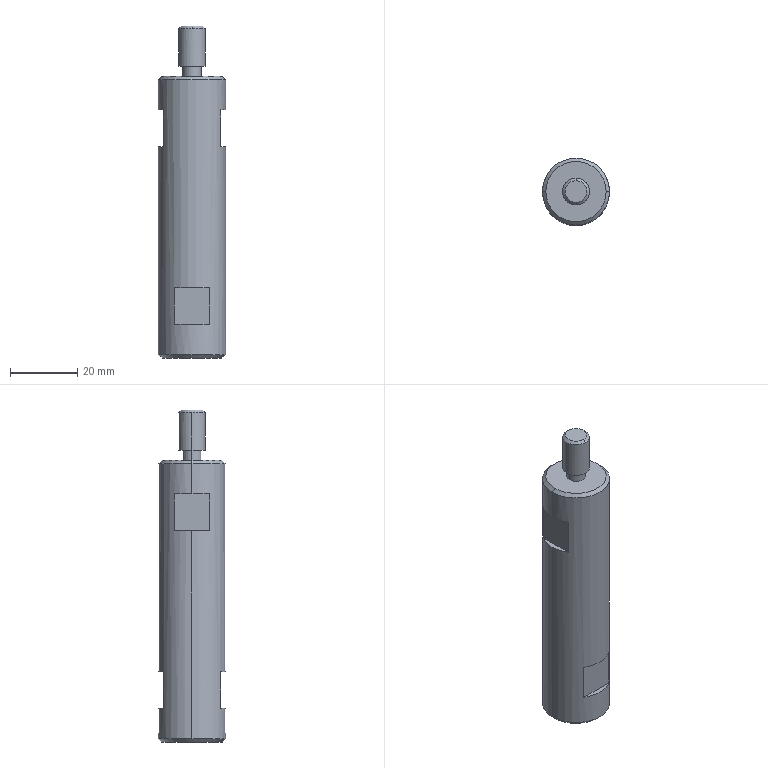Part | SolidWorks | features BaseBody 1 | 1 solid | 34 faces | box 20 x 20 x 99 mm | volume 26273 mm3 | plane 16 | cone 10 | cylinder 8 | commonest cylinder face diameters 4.917 x2 5.6 x2 8 x2 20 x2
STEP:
#1=CARTESIAN_POINT('',(-5.268,8.5,-78.));
#2=VERTEX_POINT('',#1);
#3=CARTESIAN_POINT('',(-5.268,8.5,-89.));
#4=VERTEX_POINT('',#3);
#5=CARTESIAN_POINT('',(-5.268,8.5,-50.));
#6=DIRECTION('',(0.,0.,-1.));
#7=VECTOR('',#6,1000.);
#8=LINE('',#5,#7);
#9=EDGE_CURVE('',#2,#4,#8,.T.);
#10=ORIENTED_EDGE('',*,*,#9,.T.);
#11=CARTESIAN_POINT('',(5.268,8.5,-89.));
#12=VERTEX_POINT('',#11);
#13=CARTESIAN_POINT('',(0.,0.,-89.));
#14=DIRECTION('',(0.,0.,-1.));
#15=DIRECTION('',(1.,0.,0.));
#16=AXIS2_PLACEMENT_3D('',#13,#14,#15);
#17=CIRCLE('',#16,10.);
#18=EDGE_CURVE('',#4,#12,#17,.T.);
#19=ORIENTED_EDGE('',*,*,#18,.T.);
#20=CARTESIAN_POINT('',(5.268,8.5,-78.));
#21=VERTEX_POINT('',#20);
#22=CARTESIAN_POINT('',(5.268,8.5,-50.));
#23=DIRECTION('',(0.,0.,1.));
#24=VECTOR('',#23,1000.);
#25=LINE('',#22,#24);
#26=EDGE_CURVE('',#12,#21,#25,.T.);
#27=ORIENTED_EDGE('',*,*,#26,.T.);
#28=CARTESIAN_POINT('',(0.,0.,-78.));
#29=DIRECTION('',(0.,0.,1.));
#30=DIRECTION('',(1.,0.,0.));
#31=AXIS2_PLACEMENT_3D('',#28,#29,#30);
#32=CIRCLE('',#31,10.);
#33=EDGE_CURVE('',#21,#2,#32,.T.);
#34=ORIENTED_EDGE('',*,*,#33,.T.);
#35=EDGE_LOOP('',(#10,#19,#27,#34));
#36=FACE_BOUND('',#35,.T.);
#37=CARTESIAN_POINT('',(0.,10.,-98.));
#38=VERTEX_POINT('',#37);
#39=CARTESIAN_POINT('',(-10.,0.,-98.));
#40=VERTEX_POINT('',#39);
#41=CARTESIAN_POINT('',(0.,0.,-98.));
#42=DIRECTION('',(0.,0.,1.));
#43=DIRECTION('',(1.,0.,0.));
#44=AXIS2_PLACEMENT_3D('',#41,#42,#43);
#45=CIRCLE('',#44,10.);
#46=EDGE_CURVE('',#38,#40,#45,.T.);
#47=ORIENTED_EDGE('',*,*,#46,.T.);
#48=CARTESIAN_POINT('',(-10.,0.,-36.));
#49=VERTEX_POINT('',#48);
#50=CARTESIAN_POINT('',(-10.,0.,-50.));
#51=DIRECTION('',(0.,0.,1.));
#52=VECTOR('',#51,1000.);
#53=LINE('',#50,#52);
#54=EDGE_CURVE('',#40,#49,#53,.T.);
#55=ORIENTED_EDGE('',*,*,#54,.T.);
#56=CARTESIAN_POINT('',(-8.5,5.268,-36.));
#57=VERTEX_POINT('',#56);
#58=CARTESIAN_POINT('',(0.,0.,-36.));
#59=DIRECTION('',(0.,0.,-1.));
#60=DIRECTION('',(1.,0.,0.));
#61=AXIS2_PLACEMENT_3D('',#58,#59,#60);
#62=CIRCLE('',#61,10.);
#63=EDGE_CURVE('',#49,#57,#62,.T.);
#64=ORIENTED_EDGE('',*,*,#63,.T.);
#65=CARTESIAN_POINT('',(-8.5,5.268,-25.));
#66=VERTEX_POINT('',#65);
#67=CARTESIAN_POINT('',(-8.5,5.268,-50.));
#68=DIRECTION('',(0.,0.,1.));
#69=VECTOR('',#68,1000.);
#70=LINE('',#67,#69);
#71=EDGE_CURVE('',#57,#66,#70,.T.);
#72=ORIENTED_EDGE('',*,*,#71,.T.);
#73=CARTESIAN_POINT('',(-10.,0.,-25.));
#74=VERTEX_POINT('',#73);
#75=CARTESIAN_POINT('',(0.,0.,-25.));
#76=DIRECTION('',(0.,0.,1.));
#77=DIRECTION('',(1.,0.,0.));
#78=AXIS2_PLACEMENT_3D('',#75,#76,#77);
#79=CIRCLE('',#78,10.);
#80=EDGE_CURVE('',#66,#74,#79,.T.);
#81=ORIENTED_EDGE('',*,*,#80,.T.);
#82=CARTESIAN_POINT('',(-10.,0.,-16.));
#83=VERTEX_POINT('',#82);
#84=CARTESIAN_POINT('',(-10.,0.,-50.));
#85=DIRECTION('',(0.,0.,1.));
#86=VECTOR('',#85,1000.);
#87=LINE('',#84,#86);
#88=EDGE_CURVE('',#74,#83,#87,.T.);
#89=ORIENTED_EDGE('',*,*,#88,.T.);
#90=CARTESIAN_POINT('',(10.,0.,-16.));
#91=VERTEX_POINT('',#90);
#92=CARTESIAN_POINT('',(0.,0.,-16.));
#93=DIRECTION('',(0.,0.,-1.));
#94=DIRECTION('',(1.,0.,0.));
#95=AXIS2_PLACEMENT_3D('',#92,#93,#94);
#96=CIRCLE('',#95,10.);
#97=EDGE_CURVE('',#83,#91,#96,.T.);
#98=ORIENTED_EDGE('',*,*,#97,.T.);
#99=CARTESIAN_POINT('',(10.,0.,-25.));
#100=VERTEX_POINT('',#99);
#101=CARTESIAN_POINT('',(10.,0.,-50.));
#102=DIRECTION('',(0.,0.,1.));
#103=VECTOR('',#102,1000.);
#104=LINE('',#101,#103);
#105=EDGE_CURVE('',#100,#91,#104,.T.);
#106=ORIENTED_EDGE('',*,*,#105,.F.);
#107=CARTESIAN_POINT('',(8.5,5.268,-25.));
#108=VERTEX_POINT('',#107);
#109=CARTESIAN_POINT('',(0.,0.,-25.));
#110=DIRECTION('',(0.,0.,1.));
#111=DIRECTION('',(1.,0.,0.));
#112=AXIS2_PLACEMENT_3D('',#109,#110,#111);
#113=CIRCLE('',#112,10.);
#114=EDGE_CURVE('',#100,#108,#113,.T.);
#115=ORIENTED_EDGE('',*,*,#114,.T.);
#116=CARTESIAN_POINT('',(8.5,5.268,-36.));
#117=VERTEX_POINT('',#116);
#118=CARTESIAN_POINT('',(8.5,5.268,-50.));
#119=DIRECTION('',(0.,0.,-1.));
#120=VECTOR('',#119,1000.);
#121=LINE('',#118,#120);
#122=EDGE_CURVE('',#108,#117,#121,.T.);
#123=ORIENTED_EDGE('',*,*,#122,.T.);
#124=CARTESIAN_POINT('',(10.,0.,-36.));
#125=VERTEX_POINT('',#124);
#126=CARTESIAN_POINT('',(0.,0.,-36.));
#127=DIRECTION('',(0.,0.,-1.));
#128=DIRECTION('',(1.,0.,0.));
#129=AXIS2_PLACEMENT_3D('',#126,#127,#128);
#130=CIRCLE('',#129,10.);
#131=EDGE_CURVE('',#117,#125,#130,.T.);
#132=ORIENTED_EDGE('',*,*,#131,.T.);
#133=CARTESIAN_POINT('',(10.,0.,-98.));
#134=VERTEX_POINT('',#133);
#135=CARTESIAN_POINT('',(10.,0.,-50.));
#136=DIRECTION('',(0.,0.,1.));
#137=VECTOR('',#136,1000.);
#138=LINE('',#135,#137);
#139=EDGE_CURVE('',#134,#125,#138,.T.);
#140=ORIENTED_EDGE('',*,*,#139,.F.);
#141=CARTESIAN_POINT('',(0.,0.,-98.));
#142=DIRECTION('',(0.,0.,1.));
#143=DIRECTION('',(1.,0.,0.));
#144=AXIS2_PLACEMENT_3D('',#141,#142,#143);
#145=CIRCLE('',#144,10.);
#146=EDGE_CURVE('',#134,#38,#145,.T.);
#147=ORIENTED_EDGE('',*,*,#146,.T.);
#148=EDGE_LOOP('',(#47,#55,#64,#72,#81,#89,#98,#106,#115,#123,#132,#140,#147));
#149=FACE_OUTER_BOUND('',#148,.T.);
#150=CARTESIAN_POINT('',(0.,0.,-50.));
#151=DIRECTION('',(0.,0.,1.));
#152=DIRECTION('',(1.,0.,0.));
#153=AXIS2_PLACEMENT_3D('',#150,#151,#152);
#154=CYLINDRICAL_SURFACE('',#153,10.);
#155=ADVANCED_FACE('',(#36,#149),#154,.T.);
#156=CARTESIAN_POINT('',(-9.,0.,-15.));
#157=VERTEX_POINT('',#156);
#158=CARTESIAN_POINT('',(9.,0.,-15.));
#159=VERTEX_POINT('',#158);
#160=CARTESIAN_POINT('',(0.,0.,-15.));
#161=DIRECTION('',(0.,0.,-1.));
#162=DIRECTION('',(-1.,0.,0.));
#163=AXIS2_PLACEMENT_3D('',#160,#161,#162);
#164=CIRCLE('',#163,9.);
#165=EDGE_CURVE('',#157,#159,#164,.T.);
#166=ORIENTED_EDGE('',*,*,#165,.T.);
#167=CARTESIAN_POINT('',(10.,0.,-16.));
#168=DIRECTION('',(0.7071,0.,-0.7071));
#169=VECTOR('',#168,1000.);
#170=LINE('',#167,#169);
#171=EDGE_CURVE('',#159,#91,#170,.T.);
#172=ORIENTED_EDGE('',*,*,#171,.T.);
#173=ORIENTED_EDGE('',*,*,#97,.F.);
#174=CARTESIAN_POINT('',(-10.,0.,-16.));
#175=DIRECTION('',(-0.7071,0.,-0.7071));
#176=VECTOR('',#175,1000.);
#177=LINE('',#174,#176);
#178=EDGE_CURVE('',#157,#83,#177,.T.);
#179=ORIENTED_EDGE('',*,*,#178,.F.);
#180=EDGE_LOOP('',(#166,#172,#173,#179));
#181=FACE_OUTER_BOUND('',#180,.T.);
#182=CARTESIAN_POINT('',(0.,0.,-16.));
#183=DIRECTION('',(0.,0.,-1.));
#184=DIRECTION('',(-1.,0.,0.));
#185=AXIS2_PLACEMENT_3D('',#182,#183,#184);
#186=CONICAL_SURFACE('',#185,10.,0.7854);
#187=ADVANCED_FACE('',(#181),#186,.T.);
#188=CARTESIAN_POINT('',(0.,-9.,-99.));
#189=VERTEX_POINT('',#188);
#190=CARTESIAN_POINT('',(0.,9.,-99.));
#191=VERTEX_POINT('',#190);
#192=CARTESIAN_POINT('',(0.,0.,-99.));
#193=DIRECTION('',(0.,0.,1.));
#194=DIRECTION('',(0.,-1.,0.));
#195=AXIS2_PLACEMENT_3D('',#192,#193,#194);
#196=CIRCLE('',#195,9.);
#197=EDGE_CURVE('',#189,#191,#196,.T.);
#198=ORIENTED_EDGE('',*,*,#197,.T.);
#199=CARTESIAN_POINT('',(0.,10.,-98.));
#200=DIRECTION('',(0.,0.7071,0.7071));
#201=VECTOR('',#200,1000.);
#202=LINE('',#199,#201);
#203=EDGE_CURVE('',#191,#38,#202,.T.);
#204=ORIENTED_EDGE('',*,*,#203,.T.);
#205=ORIENTED_EDGE('',*,*,#146,.F.);
#206=CARTESIAN_POINT('',(0.,-10.,-98.));
#207=VERTEX_POINT('',#206);
#208=CARTESIAN_POINT('',(0.,0.,-98.));
#209=DIRECTION('',(0.,0.,1.));
#210=DIRECTION('',(1.,0.,0.));
#211=AXIS2_PLACEMENT_3D('',#208,#209,#210);
#212=CIRCLE('',#211,10.);
#213=EDGE_CURVE('',#207,#134,#212,.T.);
#214=ORIENTED_EDGE('',*,*,#213,.F.);
#215=CARTESIAN_POINT('',(0.,-10.,-98.));
#216=DIRECTION('',(0.,-0.7071,0.7071));
#217=VECTOR('',#216,1000.);
#218=LINE('',#215,#217);
#219=EDGE_CURVE('',#189,#207,#218,.T.);
#220=ORIENTED_EDGE('',*,*,#219,.F.);
#221=EDGE_LOOP('',(#198,#204,#205,#214,#220));
#222=FACE_OUTER_BOUND('',#221,.T.);
#223=CARTESIAN_POINT('',(0.,0.,-98.));
#224=DIRECTION('',(0.,0.,1.));
#225=DIRECTION('',(0.,-1.,0.));
#226=AXIS2_PLACEMENT_3D('',#223,#224,#225);
#227=CONICAL_SURFACE('',#226,10.,0.7854);
#228=ADVANCED_FACE('',(#222),#227,.T.);
#229=CARTESIAN_POINT('',(2.8,0.,-15.));
#230=VERTEX_POINT('',#229);
#231=CARTESIAN_POINT('',(-2.8,0.,-15.));
#232=VERTEX_POINT('',#231);
#233=CARTESIAN_POINT('',(0.,0.,-15.));
#234=DIRECTION('',(0.,0.,1.));
#235=DIRECTION('',(1.,0.,0.));
#236=AXIS2_PLACEMENT_3D('',#233,#234,#235);
#237=CIRCLE('',#236,2.8);
#238=EDGE_CURVE('',#230,#232,#237,.T.);
#239=ORIENTED_EDGE('',*,*,#238,.T.);
#240=CARTESIAN_POINT('',(-2.8,0.,-12.));
#241=VERTEX_POINT('',#240);
#242=CARTESIAN_POINT('',(-2.8,0.,-50.));
#243=DIRECTION('',(0.,0.,1.));
#244=VECTOR('',#243,1000.);
#245=LINE('',#242,#244);
#246=EDGE_CURVE('',#232,#241,#245,.T.);
#247=ORIENTED_EDGE('',*,*,#246,.T.);
#248=CARTESIAN_POINT('',(2.8,0.,-12.));
#249=VERTEX_POINT('',#248);
#250=CARTESIAN_POINT('',(0.,0.,-12.));
#251=DIRECTION('',(0.,0.,-1.));
#252=DIRECTION('',(1.,0.,0.));
#253=AXIS2_PLACEMENT_3D('',#250,#251,#252);
#254=CIRCLE('',#253,2.8);
#255=EDGE_CURVE('',#241,#249,#254,.T.);
#256=ORIENTED_EDGE('',*,*,#255,.T.);
#257=CARTESIAN_POINT('',(2.8,0.,-50.));
#258=DIRECTION('',(0.,0.,1.));
#259=VECTOR('',#258,1000.);
#260=LINE('',#257,#259);
#261=EDGE_CURVE('',#230,#249,#260,.T.);
#262=ORIENTED_EDGE('',*,*,#261,.F.);
#263=EDGE_LOOP('',(#239,#247,#256,#262));
#264=FACE_OUTER_BOUND('',#263,.T.);
#265=CARTESIAN_POINT('',(0.,0.,-50.));
#266=DIRECTION('',(0.,0.,1.));
#267=DIRECTION('',(1.,0.,0.));
#268=AXIS2_PLACEMENT_3D('',#265,#266,#267);
#269=CYLINDRICAL_SURFACE('',#268,2.8);
#270=ADVANCED_FACE('',(#264),#269,.T.);
#271=CARTESIAN_POINT('',(0.,-2.458,-98.458));
#272=VERTEX_POINT('',#271);
#273=CARTESIAN_POINT('',(-2.458,0.,-98.458));
#274=VERTEX_POINT('',#273);
#275=CARTESIAN_POINT('',(0.,0.,-98.458));
#276=DIRECTION('',(0.,0.,-1.));
#277=DIRECTION('',(-1.,0.,0.));
#278=AXIS2_PLACEMENT_3D('',#275,#276,#277);
#279=CIRCLE('',#278,2.458);
#280=EDGE_CURVE('',#272,#274,#279,.T.);
#281=ORIENTED_EDGE('',*,*,#280,.F.);
#282=CARTESIAN_POINT('',(0.,-3.,-99.));
#283=VERTEX_POINT('',#282);
#284=CARTESIAN_POINT('',(0.,-3.,-99.));
#285=DIRECTION('',(0.,-0.7071,-0.7071));
#286=VECTOR('',#285,1000.);
#287=LINE('',#284,#286);
#288=EDGE_CURVE('',#272,#283,#287,.T.);
#289=ORIENTED_EDGE('',*,*,#288,.T.);
#290=CARTESIAN_POINT('',(0.,3.,-99.));
#291=VERTEX_POINT('',#290);
#292=CARTESIAN_POINT('',(0.,0.,-99.));
#293=DIRECTION('',(0.,0.,-1.));
#294=DIRECTION('',(0.,1.,0.));
#295=AXIS2_PLACEMENT_3D('',#292,#293,#294);
#296=CIRCLE('',#295,3.);
#297=EDGE_CURVE('',#283,#291,#296,.T.);
#298=ORIENTED_EDGE('',*,*,#297,.T.);
#299=CARTESIAN_POINT('',(0.,2.458,-98.458));
#300=VERTEX_POINT('',#299);
#301=CARTESIAN_POINT('',(0.,3.,-99.));
#302=DIRECTION('',(0.,0.7071,-0.7071));
#303=VECTOR('',#302,1000.);
#304=LINE('',#301,#303);
#305=EDGE_CURVE('',#300,#291,#304,.T.);
#306=ORIENTED_EDGE('',*,*,#305,.F.);
#307=CARTESIAN_POINT('',(0.,0.,-98.458));
#308=DIRECTION('',(0.,0.,-1.));
#309=DIRECTION('',(-1.,0.,0.));
#310=AXIS2_PLACEMENT_3D('',#307,#308,#309);
#311=CIRCLE('',#310,2.458);
#312=EDGE_CURVE('',#274,#300,#311,.T.);
#313=ORIENTED_EDGE('',*,*,#312,.F.);
#314=EDGE_LOOP('',(#281,#289,#298,#306,#313));
#315=FACE_OUTER_BOUND('',#314,.T.);
#316=CARTESIAN_POINT('',(0.,0.,-99.));
#317=DIRECTION('',(0.,0.,-1.));
#318=DIRECTION('',(0.,1.,0.));
#319=AXIS2_PLACEMENT_3D('',#316,#317,#318);
#320=CONICAL_SURFACE('',#319,3.,0.7854);
#321=ADVANCED_FACE('',(#315),#320,.F.);
#322=CARTESIAN_POINT('',(2.458,0.,-98.458));
#323=VERTEX_POINT('',#322);
#324=CARTESIAN_POINT('',(0.,0.,-98.458));
#325=DIRECTION('',(0.,0.,-1.));
#326=DIRECTION('',(-1.,0.,0.));
#327=AXIS2_PLACEMENT_3D('',#324,#325,#326);
#328=CIRCLE('',#327,2.458);
#329=EDGE_CURVE('',#323,#272,#328,.T.);
#330=ORIENTED_EDGE('',*,*,#329,.T.);
#331=ORIENTED_EDGE('',*,*,#280,.T.);
#332=CARTESIAN_POINT('',(-2.458,0.,-86.187));
#333=VERTEX_POINT('',#332);
#334=CARTESIAN_POINT('',(-2.458,0.,-50.));
#335=DIRECTION('',(0.,0.,1.));
#336=VECTOR('',#335,1000.);
#337=LINE('',#334,#336);
#338=EDGE_CURVE('',#274,#333,#337,.T.);
#339=ORIENTED_EDGE('',*,*,#338,.T.);
#340=CARTESIAN_POINT('',(2.458,0.,-86.187));
#341=VERTEX_POINT('',#340);
#342=CARTESIAN_POINT('',(0.,0.,-86.187));
#343=DIRECTION('',(0.,0.,-1.));
#344=DIRECTION('',(1.,0.,0.));
#345=AXIS2_PLACEMENT_3D('',#342,#343,#344);
#346=CIRCLE('',#345,2.458);
#347=EDGE_CURVE('',#341,#333,#346,.T.);
#348=ORIENTED_EDGE('',*,*,#347,.F.);
#349=CARTESIAN_POINT('',(2.458,0.,-50.));
#350=DIRECTION('',(0.,0.,1.));
#351=VECTOR('',#350,1000.);
#352=LINE('',#349,#351);
#353=EDGE_CURVE('',#323,#341,#352,.T.);
#354=ORIENTED_EDGE('',*,*,#353,.F.);
#355=EDGE_LOOP('',(#330,#331,#339,#348,#354));
#356=FACE_OUTER_BOUND('',#355,.T.);
#357=CARTESIAN_POINT('',(0.,0.,-50.));
#358=DIRECTION('',(0.,0.,1.));
#359=DIRECTION('',(1.,0.,0.));
#360=AXIS2_PLACEMENT_3D('',#357,#358,#359);
#361=CYLINDRICAL_SURFACE('',#360,2.458);
#362=ADVANCED_FACE('',(#356),#361,.F.);
#363=CARTESIAN_POINT('',(4.,0.,-12.));
#364=VERTEX_POINT('',#363);
#365=CARTESIAN_POINT('',(-4.,0.,-12.));
#366=VERTEX_POINT('',#365);
#367=CARTESIAN_POINT('',(0.,0.,-12.));
#368=DIRECTION('',(0.,0.,1.));
#369=DIRECTION('',(1.,0.,0.));
#370=AXIS2_PLACEMENT_3D('',#367,#368,#369);
#371=CIRCLE('',#370,4.);
#372=EDGE_CURVE('',#364,#366,#371,.T.);
#373=ORIENTED_EDGE('',*,*,#372,.T.);
#374=CARTESIAN_POINT('',(-4.,0.,-0.767));
#375=VERTEX_POINT('',#374);
#376=CARTESIAN_POINT('',(-4.,0.,-50.));
#377=DIRECTION('',(0.,0.,1.));
#378=VECTOR('',#377,1000.);
#379=LINE('',#376,#378);
#380=EDGE_CURVE('',#366,#375,#379,.T.);
#381=ORIENTED_EDGE('',*,*,#380,.T.);
#382=CARTESIAN_POINT('',(0.,4.,-0.767));
#383=VERTEX_POINT('',#382);
#384=CARTESIAN_POINT('',(0.,0.,-0.767));
#385=DIRECTION('',(0.,0.,-1.));
#386=DIRECTION('',(1.,0.,0.));
#387=AXIS2_PLACEMENT_3D('',#384,#385,#386);
#388=CIRCLE('',#387,4.);
#389=EDGE_CURVE('',#375,#383,#388,.T.);
#390=ORIENTED_EDGE('',*,*,#389,.T.);
#391=CARTESIAN_POINT('',(4.,0.,-0.767));
#392=VERTEX_POINT('',#391);
#393=CARTESIAN_POINT('',(0.,0.,-0.767));
#394=DIRECTION('',(0.,0.,-1.));
#395=DIRECTION('',(1.,0.,0.));
#396=AXIS2_PLACEMENT_3D('',#393,#394,#395);
#397=CIRCLE('',#396,4.);
#398=EDGE_CURVE('',#383,#392,#397,.T.);
#399=ORIENTED_EDGE('',*,*,#398,.T.);
#400=CARTESIAN_POINT('',(4.,0.,-50.));
#401=DIRECTION('',(0.,0.,1.));
#402=VECTOR('',#401,1000.);
#403=LINE('',#400,#402);
#404=EDGE_CURVE('',#364,#392,#403,.T.);
#405=ORIENTED_EDGE('',*,*,#404,.F.);
#406=EDGE_LOOP('',(#373,#381,#390,#399,#405));
#407=FACE_OUTER_BOUND('',#406,.T.);
#408=CARTESIAN_POINT('',(0.,0.,-50.));
#409=DIRECTION('',(0.,0.,1.));
#410=DIRECTION('',(1.,0.,0.));
#411=AXIS2_PLACEMENT_3D('',#408,#409,#410);
#412=CYLINDRICAL_SURFACE('',#411,4.);
#413=ADVANCED_FACE('',(#407),#412,.T.);
#414=CARTESIAN_POINT('',(0.,0.,-84.768));
#415=VERTEX_POINT('',#414);
#416=CARTESIAN_POINT('',(-2.458,0.,-86.187));
#417=DIRECTION('',(-0.866,0.,-0.5));
#418=VECTOR('',#417,1000.);
#419=LINE('',#416,#418);
#420=EDGE_CURVE('',#415,#333,#419,.T.);
#421=ORIENTED_EDGE('',*,*,#420,.F.);
#422=CARTESIAN_POINT('',(2.458,0.,-86.187));
#423=DIRECTION('',(0.866,0.,-0.5));
#424=VECTOR('',#423,1000.);
#425=LINE('',#422,#424);
#426=EDGE_CURVE('',#415,#341,#425,.T.);
#427=ORIENTED_EDGE('',*,*,#426,.T.);
#428=ORIENTED_EDGE('',*,*,#347,.T.);
#429=EDGE_LOOP('',(#421,#427,#428));
#430=FACE_OUTER_BOUND('',#429,.T.);
#431=CARTESIAN_POINT('',(0.,0.,-86.187));
#432=DIRECTION('',(0.,0.,-1.));
#433=DIRECTION('',(-1.,0.,0.));
#434=AXIS2_PLACEMENT_3D('',#431,#432,#433);
#435=CONICAL_SURFACE('',#434,2.458,1.047);
#436=ADVANCED_FACE('',(#430),#435,.F.);
#437=CARTESIAN_POINT('',(0.,3.233,0.));
#438=VERTEX_POINT('',#437);
#439=CARTESIAN_POINT('',(0.,-3.233,0.));
#440=VERTEX_POINT('',#439);
#441=CARTESIAN_POINT('',(0.,0.,0.));
#442=DIRECTION('',(0.,0.,-1.));
#443=DIRECTION('',(0.,1.,0.));
#444=AXIS2_PLACEMENT_3D('',#441,#442,#443);
#445=CIRCLE('',#444,3.233);
#446=EDGE_CURVE('',#438,#440,#445,.T.);
#447=ORIENTED_EDGE('',*,*,#446,.T.);
#448=CARTESIAN_POINT('',(0.,-4.,-0.767));
#449=VERTEX_POINT('',#448);
#450=CARTESIAN_POINT('',(0.,-4.,-0.767));
#451=DIRECTION('',(0.,-0.7071,-0.7071));
#452=VECTOR('',#451,1000.);
#453=LINE('',#450,#452);
#454=EDGE_CURVE('',#440,#449,#453,.T.);
#455=ORIENTED_EDGE('',*,*,#454,.T.);
#456=CARTESIAN_POINT('',(0.,0.,-0.767));
#457=DIRECTION('',(0.,0.,-1.));
#458=DIRECTION('',(1.,0.,0.));
#459=AXIS2_PLACEMENT_3D('',#456,#457,#458);
#460=CIRCLE('',#459,4.);
#461=EDGE_CURVE('',#392,#449,#460,.T.);
#462=ORIENTED_EDGE('',*,*,#461,.F.);
#463=ORIENTED_EDGE('',*,*,#398,.F.);
#464=CARTESIAN_POINT('',(0.,4.,-0.767));
#465=DIRECTION('',(0.,0.7071,-0.7071));
#466=VECTOR('',#465,1000.);
#467=LINE('',#464,#466);
#468=EDGE_CURVE('',#438,#383,#467,.T.);
#469=ORIENTED_EDGE('',*,*,#468,.F.);
#470=EDGE_LOOP('',(#447,#455,#462,#463,#469));
#471=FACE_OUTER_BOUND('',#470,.T.);
#472=CARTESIAN_POINT('',(0.,0.,-0.767));
#473=DIRECTION('',(0.,0.,-1.));
#474=DIRECTION('',(0.,1.,0.));
#475=AXIS2_PLACEMENT_3D('',#472,#473,#474);
#476=CONICAL_SURFACE('',#475,4.,0.7854);
#477=ADVANCED_FACE('',(#471),#476,.T.);
#478=ORIENTED_EDGE('',*,*,#54,.F.);
#479=CARTESIAN_POINT('',(0.,0.,-98.));
#480=DIRECTION('',(0.,0.,1.));
#481=DIRECTION('',(1.,0.,0.));
#482=AXIS2_PLACEMENT_3D('',#479,#480,#481);
#483=CIRCLE('',#482,10.);
#484=EDGE_CURVE('',#40,#207,#483,.T.);
#485=ORIENTED_EDGE('',*,*,#484,.T.);
#486=ORIENTED_EDGE('',*,*,#213,.T.);
#487=ORIENTED_EDGE('',*,*,#139,.T.);
#488=CARTESIAN_POINT('',(8.5,-5.268,-36.));
#489=VERTEX_POINT('',#488);
#490=CARTESIAN_POINT('',(0.,0.,-36.));
#491=DIRECTION('',(0.,0.,-1.));
#492=DIRECTION('',(1.,0.,0.));
#493=AXIS2_PLACEMENT_3D('',#490,#491,#492);
#494=CIRCLE('',#493,10.);
#495=EDGE_CURVE('',#125,#489,#494,.T.);
#496=ORIENTED_EDGE('',*,*,#495,.T.);
#497=CARTESIAN_POINT('',(8.5,-5.268,-25.));
#498=VERTEX_POINT('',#497);
#499=CARTESIAN_POINT('',(8.5,-5.268,-50.));
#500=DIRECTION('',(0.,0.,1.));
#501=VECTOR('',#500,1000.);
#502=LINE('',#499,#501);
#503=EDGE_CURVE('',#489,#498,#502,.T.);
#504=ORIENTED_EDGE('',*,*,#503,.T.);
#505=CARTESIAN_POINT('',(0.,0.,-25.));
#506=DIRECTION('',(0.,0.,1.));
#507=DIRECTION('',(1.,0.,0.));
#508=AXIS2_PLACEMENT_3D('',#505,#506,#507);
#509=CIRCLE('',#508,10.);
#510=EDGE_CURVE('',#498,#100,#509,.T.);
#511=ORIENTED_EDGE('',*,*,#510,.T.);
#512=ORIENTED_EDGE('',*,*,#105,.T.);
#513=CARTESIAN_POINT('',(0.,0.,-16.));
#514=DIRECTION('',(0.,0.,-1.));
#515=DIRECTION('',(1.,0.,0.));
#516=AXIS2_PLACEMENT_3D('',#513,#514,#515);
#517=CIRCLE('',#516,10.);
#518=EDGE_CURVE('',#91,#83,#517,.T.);
#519=ORIENTED_EDGE('',*,*,#518,.T.);
#520=ORIENTED_EDGE('',*,*,#88,.F.);
#521=CARTESIAN_POINT('',(-8.5,-5.268,-25.));
#522=VERTEX_POINT('',#521);
#523=CARTESIAN_POINT('',(0.,0.,-25.));
#524=DIRECTION('',(0.,0.,1.));
#525=DIRECTION('',(1.,0.,0.));
#526=AXIS2_PLACEMENT_3D('',#523,#524,#525);
#527=CIRCLE('',#526,10.);
#528=EDGE_CURVE('',#74,#522,#527,.T.);
#529=ORIENTED_EDGE('',*,*,#528,.T.);
#530=CARTESIAN_POINT('',(-8.5,-5.268,-36.));
#531=VERTEX_POINT('',#530);
#532=CARTESIAN_POINT('',(-8.5,-5.268,-50.));
#533=DIRECTION('',(0.,0.,-1.));
#534=VECTOR('',#533,1000.);
#535=LINE('',#532,#534);
#536=EDGE_CURVE('',#522,#531,#535,.T.);
#537=ORIENTED_EDGE('',*,*,#536,.T.);
#538=CARTESIAN_POINT('',(0.,0.,-36.));
#539=DIRECTION('',(0.,0.,-1.));
#540=DIRECTION('',(1.,0.,0.));
#541=AXIS2_PLACEMENT_3D('',#538,#539,#540);
#542=CIRCLE('',#541,10.);
#543=EDGE_CURVE('',#531,#49,#542,.T.);
#544=ORIENTED_EDGE('',*,*,#543,.T.);
#545=EDGE_LOOP('',(#478,#485,#486,#487,#496,#504,#511,#512,#519,#520,#529,#537,#544));
#546=FACE_OUTER_BOUND('',#545,.T.);
#547=CARTESIAN_POINT('',(5.268,-8.5,-78.));
#548=VERTEX_POINT('',#547);
#549=CARTESIAN_POINT('',(5.268,-8.5,-89.));
#550=VERTEX_POINT('',#549);
#551=CARTESIAN_POINT('',(5.268,-8.5,-50.));
#552=DIRECTION('',(0.,0.,-1.));
#553=VECTOR('',#552,1000.);
#554=LINE('',#551,#553);
#555=EDGE_CURVE('',#548,#550,#554,.T.);
#556=ORIENTED_EDGE('',*,*,#555,.T.);
#557=CARTESIAN_POINT('',(-5.268,-8.5,-89.));
#558=VERTEX_POINT('',#557);
#559=CARTESIAN_POINT('',(0.,0.,-89.));
#560=DIRECTION('',(0.,0.,-1.));
#561=DIRECTION('',(1.,0.,0.));
#562=AXIS2_PLACEMENT_3D('',#559,#560,#561);
#563=CIRCLE('',#562,10.);
#564=EDGE_CURVE('',#550,#558,#563,.T.);
#565=ORIENTED_EDGE('',*,*,#564,.T.);
#566=CARTESIAN_POINT('',(-5.268,-8.5,-78.));
#567=VERTEX_POINT('',#566);
#568=CARTESIAN_POINT('',(-5.268,-8.5,-50.));
#569=DIRECTION('',(0.,0.,1.));
#570=VECTOR('',#569,1000.);
#571=LINE('',#568,#570);
#572=EDGE_CURVE('',#558,#567,#571,.T.);
#573=ORIENTED_EDGE('',*,*,#572,.T.);
#574=CARTESIAN_POINT('',(0.,0.,-78.));
#575=DIRECTION('',(0.,0.,1.));
#576=DIRECTION('',(1.,0.,0.));
#577=AXIS2_PLACEMENT_3D('',#574,#575,#576);
#578=CIRCLE('',#577,10.);
#579=EDGE_CURVE('',#567,#548,#578,.T.);
#580=ORIENTED_EDGE('',*,*,#579,.T.);
#581=EDGE_LOOP('',(#556,#565,#573,#580));
#582=FACE_BOUND('',#581,.T.);
#583=CARTESIAN_POINT('',(0.,0.,-50.));
#584=DIRECTION('',(0.,0.,1.));
#585=DIRECTION('',(1.,0.,0.));
#586=AXIS2_PLACEMENT_3D('',#583,#584,#585);
#587=CYLINDRICAL_SURFACE('',#586,10.);
#588=ADVANCED_FACE('',(#546,#582),#587,.T.);
#589=CARTESIAN_POINT('',(8.5,-5.268,-36.));
#590=DIRECTION('',(0.,1.,0.));
#591=VECTOR('',#590,1000.);
#592=LINE('',#589,#591);
#593=EDGE_CURVE('',#489,#117,#592,.T.);
#594=ORIENTED_EDGE('',*,*,#593,.T.);
#595=ORIENTED_EDGE('',*,*,#122,.F.);
#596=CARTESIAN_POINT('',(8.5,-5.268,-25.));
#597=DIRECTION('',(0.,-1.,0.));
#598=VECTOR('',#597,1000.);
#599=LINE('',#596,#598);
#600=EDGE_CURVE('',#108,#498,#599,.T.);
#601=ORIENTED_EDGE('',*,*,#600,.T.);
#602=ORIENTED_EDGE('',*,*,#503,.F.);
#603=EDGE_LOOP('',(#594,#595,#601,#602));
#604=FACE_OUTER_BOUND('',#603,.T.);
#605=CARTESIAN_POINT('',(8.5,-5.268,-36.));
#606=DIRECTION('',(1.,0.,0.));
#607=DIRECTION('',(0.,0.,-1.));
#608=AXIS2_PLACEMENT_3D('',#605,#606,#607);
#609=PLANE('',#608);
#610=ADVANCED_FACE('',(#604),#609,.T.);
#611=ORIENTED_EDGE('',*,*,#131,.F.);
#612=ORIENTED_EDGE('',*,*,#593,.F.);
#613=ORIENTED_EDGE('',*,*,#495,.F.);
#614=EDGE_LOOP('',(#611,#612,#613));
#615=FACE_OUTER_BOUND('',#614,.T.);
#616=CARTESIAN_POINT('',(0.,0.,-36.));
#617=DIRECTION('',(0.,0.,1.));
#618=DIRECTION('',(1.,0.,0.));
#619=AXIS2_PLACEMENT_3D('',#616,#617,#618);
#620=PLANE('',#619);
#621=ADVANCED_FACE('',(#615),#620,.T.);
#622=ORIENTED_EDGE('',*,*,#510,.F.);
#623=ORIENTED_EDGE('',*,*,#600,.F.);
#624=ORIENTED_EDGE('',*,*,#114,.F.);
#625=EDGE_LOOP('',(#622,#623,#624));
#626=FACE_OUTER_BOUND('',#625,.T.);
#627=CARTESIAN_POINT('',(0.,0.,-25.));
#628=DIRECTION('',(0.,0.,1.));
#629=DIRECTION('',(1.,0.,0.));
#630=AXIS2_PLACEMENT_3D('',#627,#628,#629);
#631=PLANE('',#630);
#632=ADVANCED_FACE('',(#626),#631,.F.);
#633=CARTESIAN_POINT('',(-8.5,5.268,-36.));
#634=DIRECTION('',(0.,-1.,0.));
#635=VECTOR('',#634,1000.);
#636=LINE('',#633,#635);
#637=EDGE_CURVE('',#57,#531,#636,.T.);
#638=ORIENTED_EDGE('',*,*,#637,.T.);
#639=ORIENTED_EDGE('',*,*,#536,.F.);
#640=CARTESIAN_POINT('',(-8.5,5.268,-25.));
#641=DIRECTION('',(0.,1.,0.));
#642=VECTOR('',#641,1000.);
#643=LINE('',#640,#642);
#644=EDGE_CURVE('',#522,#66,#643,.T.);
#645=ORIENTED_EDGE('',*,*,#644,.T.);
#646=ORIENTED_EDGE('',*,*,#71,.F.);
#647=EDGE_LOOP('',(#638,#639,#645,#646));
#648=FACE_OUTER_BOUND('',#647,.T.);
#649=CARTESIAN_POINT('',(-8.5,5.268,-36.));
#650=DIRECTION('',(-1.,0.,0.));
#651=DIRECTION('',(0.,0.,1.));
#652=AXIS2_PLACEMENT_3D('',#649,#650,#651);
#653=PLANE('',#652);
#654=ADVANCED_FACE('',(#648),#653,.T.);
#655=ORIENTED_EDGE('',*,*,#80,.F.);
#656=ORIENTED_EDGE('',*,*,#644,.F.);
#657=ORIENTED_EDGE('',*,*,#528,.F.);
#658=EDGE_LOOP('',(#655,#656,#657));
#659=FACE_OUTER_BOUND('',#658,.T.);
#660=CARTESIAN_POINT('',(0.,0.,-25.));
#661=DIRECTION('',(0.,0.,1.));
#662=DIRECTION('',(1.,0.,0.));
#663=AXIS2_PLACEMENT_3D('',#660,#661,#662);
#664=PLANE('',#663);
#665=ADVANCED_FACE('',(#659),#664,.F.);
#666=ORIENTED_EDGE('',*,*,#543,.F.);
#667=ORIENTED_EDGE('',*,*,#637,.F.);
#668=ORIENTED_EDGE('',*,*,#63,.F.);
#669=EDGE_LOOP('',(#666,#667,#668));
#670=FACE_OUTER_BOUND('',#669,.T.);
#671=CARTESIAN_POINT('',(0.,0.,-36.));
#672=DIRECTION('',(0.,0.,1.));
#673=DIRECTION('',(1.,0.,0.));
#674=AXIS2_PLACEMENT_3D('',#671,#672,#673);
#675=PLANE('',#674);
#676=ADVANCED_FACE('',(#670),#675,.T.);
#677=ORIENTED_EDGE('',*,*,#171,.F.);
#678=CARTESIAN_POINT('',(0.,0.,-15.));
#679=DIRECTION('',(0.,0.,-1.));
#680=DIRECTION('',(-1.,0.,0.));
#681=AXIS2_PLACEMENT_3D('',#678,#679,#680);
#682=CIRCLE('',#681,9.);
#683=EDGE_CURVE('',#159,#157,#682,.T.);
#684=ORIENTED_EDGE('',*,*,#683,.T.);
#685=ORIENTED_EDGE('',*,*,#178,.T.);
#686=ORIENTED_EDGE('',*,*,#518,.F.);
#687=EDGE_LOOP('',(#677,#684,#685,#686));
#688=FACE_OUTER_BOUND('',#687,.T.);
#689=CARTESIAN_POINT('',(0.,0.,-16.));
#690=DIRECTION('',(0.,0.,-1.));
#691=DIRECTION('',(-1.,0.,0.));
#692=AXIS2_PLACEMENT_3D('',#689,#690,#691);
#693=CONICAL_SURFACE('',#692,10.,0.7854);
#694=ADVANCED_FACE('',(#688),#693,.T.);
#695=ORIENTED_EDGE('',*,*,#564,.F.);
#696=CARTESIAN_POINT('',(0.,-8.5,-89.));
#697=DIRECTION('',(-1.,0.,0.));
#698=VECTOR('',#697,1000.);
#699=LINE('',#696,#698);
#700=EDGE_CURVE('',#550,#558,#699,.T.);
#701=ORIENTED_EDGE('',*,*,#700,.T.);
#702=EDGE_LOOP('',(#695,#701));
#703=FACE_OUTER_BOUND('',#702,.T.);
#704=CARTESIAN_POINT('',(0.,0.,-89.));
#705=DIRECTION('',(0.,0.,1.));
#706=DIRECTION('',(1.,0.,0.));
#707=AXIS2_PLACEMENT_3D('',#704,#705,#706);
#708=PLANE('',#707);
#709=ADVANCED_FACE('',(#703),#708,.T.);
#710=ORIENTED_EDGE('',*,*,#555,.F.);
#711=CARTESIAN_POINT('',(-5.268,-8.5,-78.));
#712=DIRECTION('',(1.,0.,0.));
#713=VECTOR('',#712,1000.);
#714=LINE('',#711,#713);
#715=EDGE_CURVE('',#567,#548,#714,.T.);
#716=ORIENTED_EDGE('',*,*,#715,.F.);
#717=ORIENTED_EDGE('',*,*,#572,.F.);
#718=ORIENTED_EDGE('',*,*,#700,.F.);
#719=EDGE_LOOP('',(#710,#716,#717,#718));
#720=FACE_OUTER_BOUND('',#719,.T.);
#721=CARTESIAN_POINT('',(-5.268,-8.5,-78.));
#722=DIRECTION('',(0.,1.,0.));
#723=DIRECTION('',(0.,0.,1.));
#724=AXIS2_PLACEMENT_3D('',#721,#722,#723);
#725=PLANE('',#724);
#726=ADVANCED_FACE('',(#720),#725,.F.);
#727=ORIENTED_EDGE('',*,*,#579,.F.);
#728=ORIENTED_EDGE('',*,*,#715,.T.);
#729=EDGE_LOOP('',(#727,#728));
#730=FACE_OUTER_BOUND('',#729,.T.);
#731=CARTESIAN_POINT('',(0.,0.,-78.));
#732=DIRECTION('',(0.,0.,1.));
#733=DIRECTION('',(1.,0.,0.));
#734=AXIS2_PLACEMENT_3D('',#731,#732,#733);
#735=PLANE('',#734);
#736=ADVANCED_FACE('',(#730),#735,.F.);
#737=CARTESIAN_POINT('',(0.,8.5,-89.));
#738=DIRECTION('',(1.,0.,0.));
#739=VECTOR('',#738,1000.);
#740=LINE('',#737,#739);
#741=EDGE_CURVE('',#4,#12,#740,.T.);
#742=ORIENTED_EDGE('',*,*,#741,.T.);
#743=ORIENTED_EDGE('',*,*,#18,.F.);
#744=EDGE_LOOP('',(#742,#743));
#745=FACE_OUTER_BOUND('',#744,.T.);
#746=CARTESIAN_POINT('',(0.,0.,-89.));
#747=DIRECTION('',(0.,0.,1.));
#748=DIRECTION('',(1.,0.,0.));
#749=AXIS2_PLACEMENT_3D('',#746,#747,#748);
#750=PLANE('',#749);
#751=ADVANCED_FACE('',(#745),#750,.T.);
#752=ORIENTED_EDGE('',*,*,#9,.F.);
#753=CARTESIAN_POINT('',(5.268,8.5,-78.));
#754=DIRECTION('',(-1.,0.,0.));
#755=VECTOR('',#754,1000.);
#756=LINE('',#753,#755);
#757=EDGE_CURVE('',#21,#2,#756,.T.);
#758=ORIENTED_EDGE('',*,*,#757,.F.);
#759=ORIENTED_EDGE('',*,*,#26,.F.);
#760=ORIENTED_EDGE('',*,*,#741,.F.);
#761=EDGE_LOOP('',(#752,#758,#759,#760));
#762=FACE_OUTER_BOUND('',#761,.T.);
#763=CARTESIAN_POINT('',(5.268,8.5,-78.));
#764=DIRECTION('',(0.,-1.,0.));
#765=DIRECTION('',(0.,0.,-1.));
#766=AXIS2_PLACEMENT_3D('',#763,#764,#765);
#767=PLANE('',#766);
#768=ADVANCED_FACE('',(#762),#767,.F.);
#769=ORIENTED_EDGE('',*,*,#33,.F.);
#770=ORIENTED_EDGE('',*,*,#757,.T.);
#771=EDGE_LOOP('',(#769,#770));
#772=FACE_OUTER_BOUND('',#771,.T.);
#773=CARTESIAN_POINT('',(0.,0.,-78.));
#774=DIRECTION('',(0.,0.,1.));
#775=DIRECTION('',(1.,0.,0.));
#776=AXIS2_PLACEMENT_3D('',#773,#774,#775);
#777=PLANE('',#776);
#778=ADVANCED_FACE('',(#772),#777,.F.);
#779=ORIENTED_EDGE('',*,*,#203,.F.);
#780=CARTESIAN_POINT('',(0.,0.,-99.));
#781=DIRECTION('',(0.,0.,1.));
#782=DIRECTION('',(0.,-1.,0.));
#783=AXIS2_PLACEMENT_3D('',#780,#781,#782);
#784=CIRCLE('',#783,9.);
#785=EDGE_CURVE('',#191,#189,#784,.T.);
#786=ORIENTED_EDGE('',*,*,#785,.T.);
#787=ORIENTED_EDGE('',*,*,#219,.T.);
#788=ORIENTED_EDGE('',*,*,#484,.F.);
#789=ORIENTED_EDGE('',*,*,#46,.F.);
#790=EDGE_LOOP('',(#779,#786,#787,#788,#789));
#791=FACE_OUTER_BOUND('',#790,.T.);
#792=CARTESIAN_POINT('',(0.,0.,-98.));
#793=DIRECTION('',(0.,0.,1.));
#794=DIRECTION('',(0.,-1.,0.));
#795=AXIS2_PLACEMENT_3D('',#792,#793,#794);
#796=CONICAL_SURFACE('',#795,10.,0.7854);
#797=ADVANCED_FACE('',(#791),#796,.T.);
#798=ORIENTED_EDGE('',*,*,#238,.F.);
#799=CARTESIAN_POINT('',(0.,0.,-15.));
#800=DIRECTION('',(0.,0.,1.));
#801=DIRECTION('',(1.,0.,0.));
#802=AXIS2_PLACEMENT_3D('',#799,#800,#801);
#803=CIRCLE('',#802,2.8);
#804=EDGE_CURVE('',#232,#230,#803,.T.);
#805=ORIENTED_EDGE('',*,*,#804,.F.);
#806=EDGE_LOOP('',(#798,#805));
#807=FACE_BOUND('',#806,.T.);
#808=ORIENTED_EDGE('',*,*,#165,.F.);
#809=ORIENTED_EDGE('',*,*,#683,.F.);
#810=EDGE_LOOP('',(#808,#809));
#811=FACE_OUTER_BOUND('',#810,.T.);
#812=CARTESIAN_POINT('',(0.,2.8,-15.));
#813=DIRECTION('',(0.,0.,-1.));
#814=DIRECTION('',(-1.,0.,0.));
#815=AXIS2_PLACEMENT_3D('',#812,#813,#814);
#816=PLANE('',#815);
#817=ADVANCED_FACE('',(#807,#811),#816,.F.);
#818=ORIENTED_EDGE('',*,*,#197,.F.);
#819=ORIENTED_EDGE('',*,*,#785,.F.);
#820=EDGE_LOOP('',(#818,#819));
#821=FACE_OUTER_BOUND('',#820,.T.);
#822=CARTESIAN_POINT('',(0.,0.,-99.));
#823=DIRECTION('',(0.,0.,-1.));
#824=DIRECTION('',(0.,1.,0.));
#825=AXIS2_PLACEMENT_3D('',#822,#823,#824);
#826=CIRCLE('',#825,3.);
#827=EDGE_CURVE('',#291,#283,#826,.T.);
#828=ORIENTED_EDGE('',*,*,#827,.F.);
#829=ORIENTED_EDGE('',*,*,#297,.F.);
#830=EDGE_LOOP('',(#828,#829));
#831=FACE_BOUND('',#830,.T.);
#832=CARTESIAN_POINT('',(0.,9.,-99.));
#833=DIRECTION('',(0.,0.,1.));
#834=DIRECTION('',(1.,0.,0.));
#835=AXIS2_PLACEMENT_3D('',#832,#833,#834);
#836=PLANE('',#835);
#837=ADVANCED_FACE('',(#821,#831),#836,.F.);
#838=ORIENTED_EDGE('',*,*,#246,.F.);
#839=ORIENTED_EDGE('',*,*,#804,.T.);
#840=ORIENTED_EDGE('',*,*,#261,.T.);
#841=CARTESIAN_POINT('',(0.,0.,-12.));
#842=DIRECTION('',(0.,0.,-1.));
#843=DIRECTION('',(1.,0.,0.));
#844=AXIS2_PLACEMENT_3D('',#841,#842,#843);
#845=CIRCLE('',#844,2.8);
#846=EDGE_CURVE('',#249,#241,#845,.T.);
#847=ORIENTED_EDGE('',*,*,#846,.T.);
#848=EDGE_LOOP('',(#838,#839,#840,#847));
#849=FACE_OUTER_BOUND('',#848,.T.);
#850=CARTESIAN_POINT('',(0.,0.,-50.));
#851=DIRECTION('',(0.,0.,1.));
#852=DIRECTION('',(1.,0.,0.));
#853=AXIS2_PLACEMENT_3D('',#850,#851,#852);
#854=CYLINDRICAL_SURFACE('',#853,2.8);
#855=ADVANCED_FACE('',(#849),#854,.T.);
#856=ORIENTED_EDGE('',*,*,#288,.F.);
#857=ORIENTED_EDGE('',*,*,#329,.F.);
#858=CARTESIAN_POINT('',(0.,0.,-98.458));
#859=DIRECTION('',(0.,0.,-1.));
#860=DIRECTION('',(-1.,0.,0.));
#861=AXIS2_PLACEMENT_3D('',#858,#859,#860);
#862=CIRCLE('',#861,2.458);
#863=EDGE_CURVE('',#300,#323,#862,.T.);
#864=ORIENTED_EDGE('',*,*,#863,.F.);
#865=ORIENTED_EDGE('',*,*,#305,.T.);
#866=ORIENTED_EDGE('',*,*,#827,.T.);
#867=EDGE_LOOP('',(#856,#857,#864,#865,#866));
#868=FACE_OUTER_BOUND('',#867,.T.);
#869=CARTESIAN_POINT('',(0.,0.,-99.));
#870=DIRECTION('',(0.,0.,-1.));
#871=DIRECTION('',(0.,1.,0.));
#872=AXIS2_PLACEMENT_3D('',#869,#870,#871);
#873=CONICAL_SURFACE('',#872,3.,0.7854);
#874=ADVANCED_FACE('',(#868),#873,.F.);
#875=ORIENTED_EDGE('',*,*,#372,.F.);
#876=CARTESIAN_POINT('',(0.,0.,-12.));
#877=DIRECTION('',(0.,0.,1.));
#878=DIRECTION('',(1.,0.,0.));
#879=AXIS2_PLACEMENT_3D('',#876,#877,#878);
#880=CIRCLE('',#879,4.);
#881=EDGE_CURVE('',#366,#364,#880,.T.);
#882=ORIENTED_EDGE('',*,*,#881,.F.);
#883=EDGE_LOOP('',(#875,#882));
#884=FACE_OUTER_BOUND('',#883,.T.);
#885=ORIENTED_EDGE('',*,*,#846,.F.);
#886=ORIENTED_EDGE('',*,*,#255,.F.);
#887=EDGE_LOOP('',(#885,#886));
#888=FACE_BOUND('',#887,.T.);
#889=CARTESIAN_POINT('',(0.,4.,-12.));
#890=DIRECTION('',(0.,0.,1.));
#891=DIRECTION('',(1.,0.,0.));
#892=AXIS2_PLACEMENT_3D('',#889,#890,#891);
#893=PLANE('',#892);
#894=ADVANCED_FACE('',(#884,#888),#893,.F.);
#895=ORIENTED_EDGE('',*,*,#338,.F.);
#896=ORIENTED_EDGE('',*,*,#312,.T.);
#897=ORIENTED_EDGE('',*,*,#863,.T.);
#898=ORIENTED_EDGE('',*,*,#353,.T.);
#899=CARTESIAN_POINT('',(0.,0.,-86.187));
#900=DIRECTION('',(0.,0.,-1.));
#901=DIRECTION('',(1.,0.,0.));
#902=AXIS2_PLACEMENT_3D('',#899,#900,#901);
#903=CIRCLE('',#902,2.458);
#904=EDGE_CURVE('',#333,#341,#903,.T.);
#905=ORIENTED_EDGE('',*,*,#904,.F.);
#906=EDGE_LOOP('',(#895,#896,#897,#898,#905));
#907=FACE_OUTER_BOUND('',#906,.T.);
#908=CARTESIAN_POINT('',(0.,0.,-50.));
#909=DIRECTION('',(0.,0.,1.));
#910=DIRECTION('',(1.,0.,0.));
#911=AXIS2_PLACEMENT_3D('',#908,#909,#910);
#912=CYLINDRICAL_SURFACE('',#911,2.458);
#913=ADVANCED_FACE('',(#907),#912,.F.);
#914=ORIENTED_EDGE('',*,*,#380,.F.);
#915=ORIENTED_EDGE('',*,*,#881,.T.);
#916=ORIENTED_EDGE('',*,*,#404,.T.);
#917=ORIENTED_EDGE('',*,*,#461,.T.);
#918=CARTESIAN_POINT('',(0.,0.,-0.767));
#919=DIRECTION('',(0.,0.,-1.));
#920=DIRECTION('',(1.,0.,0.));
#921=AXIS2_PLACEMENT_3D('',#918,#919,#920);
#922=CIRCLE('',#921,4.);
#923=EDGE_CURVE('',#449,#375,#922,.T.);
#924=ORIENTED_EDGE('',*,*,#923,.T.);
#925=EDGE_LOOP('',(#914,#915,#916,#917,#924));
#926=FACE_OUTER_BOUND('',#925,.T.);
#927=CARTESIAN_POINT('',(0.,0.,-50.));
#928=DIRECTION('',(0.,0.,1.));
#929=DIRECTION('',(1.,0.,0.));
#930=AXIS2_PLACEMENT_3D('',#927,#928,#929);
#931=CYLINDRICAL_SURFACE('',#930,4.);
#932=ADVANCED_FACE('',(#926),#931,.T.);
#933=ORIENTED_EDGE('',*,*,#426,.F.);
#934=ORIENTED_EDGE('',*,*,#420,.T.);
#935=ORIENTED_EDGE('',*,*,#904,.T.);
#936=EDGE_LOOP('',(#933,#934,#935));
#937=FACE_OUTER_BOUND('',#936,.T.);
#938=CARTESIAN_POINT('',(0.,0.,-86.187));
#939=DIRECTION('',(0.,0.,-1.));
#940=DIRECTION('',(-1.,0.,0.));
#941=AXIS2_PLACEMENT_3D('',#938,#939,#940);
#942=CONICAL_SURFACE('',#941,2.458,1.047);
#943=ADVANCED_FACE('',(#937),#942,.F.);
#944=ORIENTED_EDGE('',*,*,#454,.F.);
#945=CARTESIAN_POINT('',(0.,0.,0.));
#946=DIRECTION('',(0.,0.,-1.));
#947=DIRECTION('',(0.,1.,0.));
#948=AXIS2_PLACEMENT_3D('',#945,#946,#947);
#949=CIRCLE('',#948,3.233);
#950=EDGE_CURVE('',#440,#438,#949,.T.);
#951=ORIENTED_EDGE('',*,*,#950,.T.);
#952=ORIENTED_EDGE('',*,*,#468,.T.);
#953=ORIENTED_EDGE('',*,*,#389,.F.);
#954=ORIENTED_EDGE('',*,*,#923,.F.);
#955=EDGE_LOOP('',(#944,#951,#952,#953,#954));
#956=FACE_OUTER_BOUND('',#955,.T.);
#957=CARTESIAN_POINT('',(0.,0.,-0.767));
#958=DIRECTION('',(0.,0.,-1.));
#959=DIRECTION('',(0.,1.,0.));
#960=AXIS2_PLACEMENT_3D('',#957,#958,#959);
#961=CONICAL_SURFACE('',#960,4.,0.7854);
#962=ADVANCED_FACE('',(#956),#961,.T.);
#963=ORIENTED_EDGE('',*,*,#446,.F.);
#964=ORIENTED_EDGE('',*,*,#950,.F.);
#965=EDGE_LOOP('',(#963,#964));
#966=FACE_OUTER_BOUND('',#965,.T.);
#967=CARTESIAN_POINT('',(0.,0.,0.));
#968=DIRECTION('',(0.,0.,-1.));
#969=DIRECTION('',(-1.,0.,0.));
#970=AXIS2_PLACEMENT_3D('',#967,#968,#969);
#971=PLANE('',#970);
#972=ADVANCED_FACE('',(#966),#971,.F.);
#973=CLOSED_SHELL('',(#155,#187,#228,#270,#321,#362,#413,#436,#477,#588,#610,#621,#632,#654,#665,#676,#694,#709,#726,#736,#751,#768,#778,#797,#817,#837,#855,#874,#894,#913,#932,#943,#962,#972));
#974=MANIFOLD_SOLID_BREP('',#973);
#975=CARTESIAN_POINT('',(0.,0.,0.));
#976=DIRECTION('',(0.,0.,1.));
#977=DIRECTION('',(1.,0.,0.));
#978=AXIS2_PLACEMENT_3D('',#975,#976,#977);
#979=(LENGTH_UNIT()NAMED_UNIT(*)SI_UNIT(.MILLI.,.METRE.));
#980=UNCERTAINTY_MEASURE_WITH_UNIT(LENGTH_MEASURE(0.00001),#979,'','');
#981=(NAMED_UNIT(*)PLANE_ANGLE_UNIT()SI_UNIT($,.RADIAN.));
#982=(NAMED_UNIT(*)SI_UNIT($,.STERADIAN.)SOLID_ANGLE_UNIT());
#983=(GEOMETRIC_REPRESENTATION_CONTEXT(3)GLOBAL_UNCERTAINTY_ASSIGNED_CONTEXT((#980))GLOBAL_UNIT_ASSIGNED_CONTEXT((#979,#981,#982))REPRESENTATION_CONTEXT('',''));
#984=ADVANCED_BREP_SHAPE_REPRESENTATION('',(#974,#978),#983);